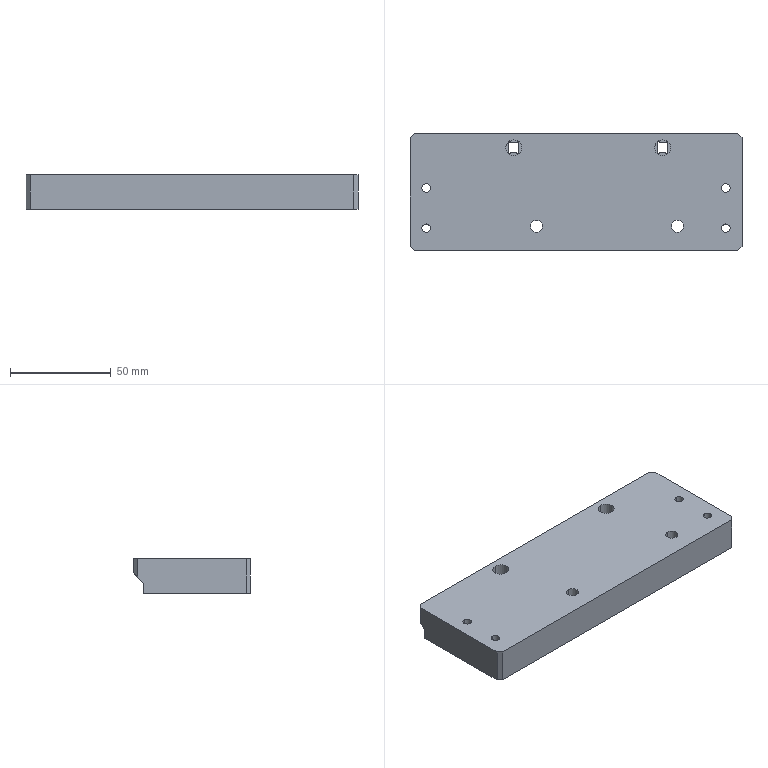NC program | NX | posted with a generic post | part box 165 x 58 x 17 mm
Lines 1 to 1651 of 3780, first 1438 of 1635 lines:
N10 G17 G21 G94 G90
(FLOOR_WALL , TOOL : D80)
N12 T19 M6
N14 G54
N16 G17 G0 G90 X127.5 Y0. S6500 M3
N18 G43 Z30. H19
N20 Z3.
N22 G94 G1 Z0. F1500.
N24 X124.5
N26 X-124.5
N28 X-127.5
N30 Z3.
N32 G0 Z30.
N34 M5
(ZLEVEL_PROFILE , TOOL : D10)
N36 T15 M6
N38 G54
N40 G17 G0 G90 X-47.703 Y34.1 S9500 M3
N42 G43 Z30. H15
N44 Z1.5
N46 G94 G1 X0. Z-1. F1000.
N48 X80.5 F3000.
N50 G2 X84.106 Y32.606 R5.1
N52 G1 X86.106 Y30.606
N54 G2 X87.6 Y27. R5.1
N56 G1 Y-27.
N58 G2 X86.106 Y-30.606 R5.1
N60 G1 X84.106 Y-32.606
N62 G2 X80.5 Y-34.1 R5.1
N64 G1 X-80.5
N66 G2 X-84.106 Y-32.606 R5.1
N68 G1 X-86.106 Y-30.606
N70 G2 X-87.6 Y-27. R5.1
N72 G1 Y27.
N74 G2 X-86.106 Y30.606 R5.1
N76 G1 X-84.106 Y32.606
N78 G2 X-80.5 Y34.1 R5.1
N80 G1 X0.
N82 X80.5 Z-1.17
N84 X81. Y34.075 Z-1.171
N86 X81.495 Y34.002 Z-1.172
N88 X81.98 Y33.88 Z-1.173
N90 X82.452 Y33.712 Z-1.174
N92 X82.904 Y33.498 Z-1.175
N94 X83.333 Y33.24 Z-1.176
N96 X83.735 Y32.942 Z-1.177
N98 X84.106 Y32.606 Z-1.179
N100 X86.106 Y30.606 Z-1.185
N102 X86.442 Y30.235 Z-1.186
N104 X86.74 Y29.833 Z-1.187
N106 X86.998 Y29.404 Z-1.188
N108 X87.212 Y28.952 Z-1.189
N110 X87.38 Y28.48 Z-1.19
N112 X87.502 Y27.995 Z-1.191
N114 X87.575 Y27.5 Z-1.192
N116 X87.6 Y27. Z-1.193
N118 Y-27. Z-1.307
N120 X87.575 Y-27.5 Z-1.308
N122 X87.502 Y-27.995 Z-1.309
N124 X87.38 Y-28.48 Z-1.31
N126 X87.212 Y-28.952 Z-1.311
N128 X86.998 Y-29.404 Z-1.312
N130 X86.74 Y-29.833 Z-1.313
N132 X86.442 Y-30.235 Z-1.314
N134 X86.106 Y-30.606 Z-1.315
N136 X84.106 Y-32.606 Z-1.321
N138 X83.735 Y-32.942 Z-1.323
N140 X83.333 Y-33.24 Z-1.324
N142 X82.904 Y-33.498 Z-1.325
N144 X82.452 Y-33.712 Z-1.326
N146 X81.98 Y-33.88 Z-1.327
N148 X81.495 Y-34.002 Z-1.328
N150 X81. Y-34.075 Z-1.329
N152 X80.5 Y-34.1 Z-1.33
N154 X-80.5 Z-1.67
N156 X-81. Y-34.075 Z-1.671
N158 X-81.495 Y-34.002 Z-1.672
N160 X-81.98 Y-33.88 Z-1.673
N162 X-82.452 Y-33.712 Z-1.674
N164 X-82.904 Y-33.498 Z-1.675
N166 X-83.333 Y-33.24 Z-1.676
N168 X-83.735 Y-32.942 Z-1.677
N170 X-84.106 Y-32.606 Z-1.679
N172 X-86.106 Y-30.606 Z-1.685
N174 X-86.442 Y-30.235 Z-1.686
N176 X-86.74 Y-29.833 Z-1.687
N178 X-86.998 Y-29.404 Z-1.688
N180 X-87.212 Y-28.952 Z-1.689
N182 X-87.38 Y-28.48 Z-1.69
N184 X-87.502 Y-27.995 Z-1.691
N186 X-87.575 Y-27.5 Z-1.692
N188 X-87.6 Y-27. Z-1.693
N190 Y27. Z-1.807
N192 X-87.575 Y27.5 Z-1.808
N194 X-87.502 Y27.995 Z-1.809
N196 X-87.38 Y28.48 Z-1.81
N198 X-87.212 Y28.952 Z-1.811
N200 X-86.998 Y29.404 Z-1.812
N202 X-86.74 Y29.833 Z-1.813
N204 X-86.442 Y30.235 Z-1.814
N206 X-86.106 Y30.606 Z-1.815
N208 X-84.106 Y32.606 Z-1.821
N210 X-83.735 Y32.942 Z-1.823
N212 X-83.333 Y33.24 Z-1.824
N214 X-82.904 Y33.498 Z-1.825
N216 X-82.452 Y33.712 Z-1.826
N218 X-81.98 Y33.88 Z-1.827
N220 X-81.495 Y34.002 Z-1.828
N222 X-81. Y34.075 Z-1.829
N224 X-80.5 Y34.1 Z-1.83
N226 X0. Z-2.
N228 X80.5 Z-2.17
N230 X81. Y34.075 Z-2.171
N232 X81.495 Y34.002 Z-2.172
N234 X81.98 Y33.88 Z-2.173
N236 X82.452 Y33.712 Z-2.174
N238 X82.904 Y33.498 Z-2.175
N240 X83.333 Y33.24 Z-2.176
N242 X83.735 Y32.942 Z-2.177
N244 X84.106 Y32.606 Z-2.179
N246 X86.106 Y30.606 Z-2.185
N248 X86.442 Y30.235 Z-2.186
N250 X86.74 Y29.833 Z-2.187
N252 X86.998 Y29.404 Z-2.188
N254 X87.212 Y28.952 Z-2.189
N256 X87.38 Y28.48 Z-2.19
N258 X87.502 Y27.995 Z-2.191
N260 X87.575 Y27.5 Z-2.192
N262 X87.6 Y27. Z-2.193
N264 Y-27. Z-2.307
N266 X87.575 Y-27.5 Z-2.308
N268 X87.502 Y-27.995 Z-2.309
N270 X87.38 Y-28.48 Z-2.31
N272 X87.212 Y-28.952 Z-2.311
N274 X86.998 Y-29.404 Z-2.312
N276 X86.74 Y-29.833 Z-2.313
N278 X86.442 Y-30.235 Z-2.314
N280 X86.106 Y-30.606 Z-2.315
N282 X84.106 Y-32.606 Z-2.321
N284 X83.735 Y-32.942 Z-2.323
N286 X83.333 Y-33.24 Z-2.324
N288 X82.904 Y-33.498 Z-2.325
N290 X82.452 Y-33.712 Z-2.326
N292 X81.98 Y-33.88 Z-2.327
N294 X81.495 Y-34.002 Z-2.328
N296 X81. Y-34.075 Z-2.329
N298 X80.5 Y-34.1 Z-2.33
N300 X-80.5 Z-2.67
N302 X-81. Y-34.075 Z-2.671
N304 X-81.495 Y-34.002 Z-2.672
N306 X-81.98 Y-33.88 Z-2.673
N308 X-82.452 Y-33.712 Z-2.674
N310 X-82.904 Y-33.498 Z-2.675
N312 X-83.333 Y-33.24 Z-2.676
N314 X-83.735 Y-32.942 Z-2.677
N316 X-84.106 Y-32.606 Z-2.679
N318 X-86.106 Y-30.606 Z-2.685
N320 X-86.442 Y-30.235 Z-2.686
N322 X-86.74 Y-29.833 Z-2.687
N324 X-86.998 Y-29.404 Z-2.688
N326 X-87.212 Y-28.952 Z-2.689
N328 X-87.38 Y-28.48 Z-2.69
N330 X-87.502 Y-27.995 Z-2.691
N332 X-87.575 Y-27.5 Z-2.692
N334 X-87.6 Y-27. Z-2.693
N336 Y27. Z-2.807
N338 X-87.575 Y27.5 Z-2.808
N340 X-87.502 Y27.995 Z-2.809
N342 X-87.38 Y28.48 Z-2.81
N344 X-87.212 Y28.952 Z-2.811
N346 X-86.998 Y29.404 Z-2.812
N348 X-86.74 Y29.833 Z-2.813
N350 X-86.442 Y30.235 Z-2.814
N352 X-86.106 Y30.606 Z-2.815
N354 X-84.106 Y32.606 Z-2.821
N356 X-83.735 Y32.942 Z-2.823
N358 X-83.333 Y33.24 Z-2.824
N360 X-82.904 Y33.498 Z-2.825
N362 X-82.452 Y33.712 Z-2.826
N364 X-81.98 Y33.88 Z-2.827
N366 X-81.495 Y34.002 Z-2.828
N368 X-81. Y34.075 Z-2.829
N370 X-80.5 Y34.1 Z-2.83
N372 X0. Z-3.
N374 X80.5 Z-3.17
N376 X81. Y34.075 Z-3.171
N378 X81.495 Y34.002 Z-3.172
N380 X81.98 Y33.88 Z-3.173
N382 X82.452 Y33.712 Z-3.174
N384 X82.904 Y33.498 Z-3.175
N386 X83.333 Y33.24 Z-3.176
N388 X83.735 Y32.942 Z-3.177
N390 X84.106 Y32.606 Z-3.179
N392 X86.106 Y30.606 Z-3.185
N394 X86.442 Y30.235 Z-3.186
N396 X86.74 Y29.833 Z-3.187
N398 X86.998 Y29.404 Z-3.188
N400 X87.212 Y28.952 Z-3.189
N402 X87.38 Y28.48 Z-3.19
N404 X87.502 Y27.995 Z-3.191
N406 X87.575 Y27.5 Z-3.192
N408 X87.6 Y27. Z-3.193
N410 Y-27. Z-3.307
N412 X87.575 Y-27.5 Z-3.308
N414 X87.502 Y-27.995 Z-3.309
N416 X87.38 Y-28.48 Z-3.31
N418 X87.212 Y-28.952 Z-3.311
N420 X86.998 Y-29.404 Z-3.312
N422 X86.74 Y-29.833 Z-3.313
N424 X86.442 Y-30.235 Z-3.314
N426 X86.106 Y-30.606 Z-3.315
N428 X84.106 Y-32.606 Z-3.321
N430 X83.735 Y-32.942 Z-3.323
N432 X83.333 Y-33.24 Z-3.324
N434 X82.904 Y-33.498 Z-3.325
N436 X82.452 Y-33.712 Z-3.326
N438 X81.98 Y-33.88 Z-3.327
N440 X81.495 Y-34.002 Z-3.328
N442 X81. Y-34.075 Z-3.329
N444 X80.5 Y-34.1 Z-3.33
N446 X-80.5 Z-3.67
N448 X-81. Y-34.075 Z-3.671
N450 X-81.495 Y-34.002 Z-3.672
N452 X-81.98 Y-33.88 Z-3.673
N454 X-82.452 Y-33.712 Z-3.674
N456 X-82.904 Y-33.498 Z-3.675
N458 X-83.333 Y-33.24 Z-3.676
N460 X-83.735 Y-32.942 Z-3.677
N462 X-84.106 Y-32.606 Z-3.679
N464 X-86.106 Y-30.606 Z-3.685
N466 X-86.442 Y-30.235 Z-3.686
N468 X-86.74 Y-29.833 Z-3.687
N470 X-86.998 Y-29.404 Z-3.688
N472 X-87.212 Y-28.952 Z-3.689
N474 X-87.38 Y-28.48 Z-3.69
N476 X-87.502 Y-27.995 Z-3.691
N478 X-87.575 Y-27.5 Z-3.692
N480 X-87.6 Y-27. Z-3.693
N482 Y27. Z-3.807
N484 X-87.575 Y27.5 Z-3.808
N486 X-87.502 Y27.995 Z-3.809
N488 X-87.38 Y28.48 Z-3.81
N490 X-87.212 Y28.952 Z-3.811
N492 X-86.998 Y29.404 Z-3.812
N494 X-86.74 Y29.833 Z-3.813
N496 X-86.442 Y30.235 Z-3.814
N498 X-86.106 Y30.606 Z-3.815
N500 X-84.106 Y32.606 Z-3.821
N502 X-83.735 Y32.942 Z-3.823
N504 X-83.333 Y33.24 Z-3.824
N506 X-82.904 Y33.498 Z-3.825
N508 X-82.452 Y33.712 Z-3.826
N510 X-81.98 Y33.88 Z-3.827
N512 X-81.495 Y34.002 Z-3.828
N514 X-81. Y34.075 Z-3.829
N516 X-80.5 Y34.1 Z-3.83
N518 X0. Z-4.
N520 X80.5 Z-4.17
N522 X81. Y34.075 Z-4.171
N524 X81.495 Y34.002 Z-4.172
N526 X81.98 Y33.88 Z-4.173
N528 X82.452 Y33.712 Z-4.174
N530 X82.904 Y33.498 Z-4.175
N532 X83.333 Y33.24 Z-4.176
N534 X83.735 Y32.942 Z-4.177
N536 X84.106 Y32.606 Z-4.179
N538 X86.106 Y30.606 Z-4.185
N540 X86.442 Y30.235 Z-4.186
N542 X86.74 Y29.833 Z-4.187
N544 X86.998 Y29.404 Z-4.188
N546 X87.212 Y28.952 Z-4.189
N548 X87.38 Y28.48 Z-4.19
N550 X87.502 Y27.995 Z-4.191
N552 X87.575 Y27.5 Z-4.192
N554 X87.6 Y27. Z-4.193
N556 Y-27. Z-4.307
N558 X87.575 Y-27.5 Z-4.308
N560 X87.502 Y-27.995 Z-4.309
N562 X87.38 Y-28.48 Z-4.31
N564 X87.212 Y-28.952 Z-4.311
N566 X86.998 Y-29.404 Z-4.312
N568 X86.74 Y-29.833 Z-4.313
N570 X86.442 Y-30.235 Z-4.314
N572 X86.106 Y-30.606 Z-4.315
N574 X84.106 Y-32.606 Z-4.321
N576 X83.735 Y-32.942 Z-4.323
N578 X83.333 Y-33.24 Z-4.324
N580 X82.904 Y-33.498 Z-4.325
N582 X82.452 Y-33.712 Z-4.326
N584 X81.98 Y-33.88 Z-4.327
N586 X81.495 Y-34.002 Z-4.328
N588 X81. Y-34.075 Z-4.329
N590 X80.5 Y-34.1 Z-4.33
N592 X-80.5 Z-4.67
N594 X-81. Y-34.075 Z-4.671
N596 X-81.495 Y-34.002 Z-4.672
N598 X-81.98 Y-33.88 Z-4.673
N600 X-82.452 Y-33.712 Z-4.674
N602 X-82.904 Y-33.498 Z-4.675
N604 X-83.333 Y-33.24 Z-4.676
N606 X-83.735 Y-32.942 Z-4.677
N608 X-84.106 Y-32.606 Z-4.679
N610 X-86.106 Y-30.606 Z-4.685
N612 X-86.442 Y-30.235 Z-4.686
N614 X-86.74 Y-29.833 Z-4.687
N616 X-86.998 Y-29.404 Z-4.688
N618 X-87.212 Y-28.952 Z-4.689
N620 X-87.38 Y-28.48 Z-4.69
N622 X-87.502 Y-27.995 Z-4.691
N624 X-87.575 Y-27.5 Z-4.692
N626 X-87.6 Y-27. Z-4.693
N628 Y27. Z-4.807
N630 X-87.575 Y27.5 Z-4.808
N632 X-87.502 Y27.995 Z-4.809
N634 X-87.38 Y28.48 Z-4.81
N636 X-87.212 Y28.952 Z-4.811
N638 X-86.998 Y29.404 Z-4.812
N640 X-86.74 Y29.833 Z-4.813
N642 X-86.442 Y30.235 Z-4.814
N644 X-86.106 Y30.606 Z-4.815
N646 X-84.106 Y32.606 Z-4.821
N648 X-83.735 Y32.942 Z-4.823
N650 X-83.333 Y33.24 Z-4.824
N652 X-82.904 Y33.498 Z-4.825
N654 X-82.452 Y33.712 Z-4.826
N656 X-81.98 Y33.88 Z-4.827
N658 X-81.495 Y34.002 Z-4.828
N660 X-81. Y34.075 Z-4.829
N662 X-80.5 Y34.1 Z-4.83
N664 X0. Z-5.
N666 X80.5 Z-5.17
N668 X81. Y34.075 Z-5.171
N670 X81.495 Y34.002 Z-5.172
N672 X81.98 Y33.88 Z-5.173
N674 X82.452 Y33.712 Z-5.174
N676 X82.904 Y33.498 Z-5.175
N678 X83.333 Y33.24 Z-5.176
N680 X83.735 Y32.942 Z-5.177
N682 X84.106 Y32.606 Z-5.179
N684 X86.106 Y30.606 Z-5.185
N686 X86.442 Y30.235 Z-5.186
N688 X86.74 Y29.833 Z-5.187
N690 X86.998 Y29.404 Z-5.188
N692 X87.212 Y28.952 Z-5.189
N694 X87.38 Y28.48 Z-5.19
N696 X87.502 Y27.995 Z-5.191
N698 X87.575 Y27.5 Z-5.192
N700 X87.6 Y27. Z-5.193
N702 Y-27. Z-5.307
N704 X87.575 Y-27.5 Z-5.308
N706 X87.502 Y-27.995 Z-5.309
N708 X87.38 Y-28.48 Z-5.31
N710 X87.212 Y-28.952 Z-5.311
N712 X86.998 Y-29.404 Z-5.312
N714 X86.74 Y-29.833 Z-5.313
N716 X86.442 Y-30.235 Z-5.314
N718 X86.106 Y-30.606 Z-5.315
N720 X84.106 Y-32.606 Z-5.321
N722 X83.735 Y-32.942 Z-5.323
N724 X83.333 Y-33.24 Z-5.324
N726 X82.904 Y-33.498 Z-5.325
N728 X82.452 Y-33.712 Z-5.326
N730 X81.98 Y-33.88 Z-5.327
N732 X81.495 Y-34.002 Z-5.328
N734 X81. Y-34.075 Z-5.329
N736 X80.5 Y-34.1 Z-5.33
N738 X-80.5 Z-5.67
N740 X-81. Y-34.075 Z-5.671
N742 X-81.495 Y-34.002 Z-5.672
N744 X-81.98 Y-33.88 Z-5.673
N746 X-82.452 Y-33.712 Z-5.674
N748 X-82.904 Y-33.498 Z-5.675
N750 X-83.333 Y-33.24 Z-5.676
N752 X-83.735 Y-32.942 Z-5.677
N754 X-84.106 Y-32.606 Z-5.679
N756 X-86.106 Y-30.606 Z-5.685
N758 X-86.442 Y-30.235 Z-5.686
N760 X-86.74 Y-29.833 Z-5.687
N762 X-86.998 Y-29.404 Z-5.688
N764 X-87.212 Y-28.952 Z-5.689
N766 X-87.38 Y-28.48 Z-5.69
N768 X-87.502 Y-27.995 Z-5.691
N770 X-87.575 Y-27.5 Z-5.692
N772 X-87.6 Y-27. Z-5.693
N774 Y27. Z-5.807
N776 X-87.575 Y27.5 Z-5.808
N778 X-87.502 Y27.995 Z-5.809
N780 X-87.38 Y28.48 Z-5.81
N782 X-87.212 Y28.952 Z-5.811
N784 X-86.998 Y29.404 Z-5.812
N786 X-86.74 Y29.833 Z-5.813
N788 X-86.442 Y30.235 Z-5.814
N790 X-86.106 Y30.606 Z-5.815
N792 X-84.106 Y32.606 Z-5.821
N794 X-83.735 Y32.942 Z-5.823
N796 X-83.333 Y33.24 Z-5.824
N798 X-82.904 Y33.498 Z-5.825
N800 X-82.452 Y33.712 Z-5.826
N802 X-81.98 Y33.88 Z-5.827
N804 X-81.495 Y34.002 Z-5.828
N806 X-81. Y34.075 Z-5.829
N808 X-80.5 Y34.1 Z-5.83
N810 X0. Z-6.
N812 X80.5 Z-6.17
N814 X81. Y34.075 Z-6.171
N816 X81.495 Y34.002 Z-6.172
N818 X81.98 Y33.88 Z-6.173
N820 X82.452 Y33.712 Z-6.174
N822 X82.904 Y33.498 Z-6.175
N824 X83.333 Y33.24 Z-6.176
N826 X83.735 Y32.942 Z-6.177
N828 X84.106 Y32.606 Z-6.179
N830 X86.106 Y30.606 Z-6.185
N832 X86.442 Y30.235 Z-6.186
N834 X86.74 Y29.833 Z-6.187
N836 X86.998 Y29.404 Z-6.188
N838 X87.212 Y28.952 Z-6.189
N840 X87.38 Y28.48 Z-6.19
N842 X87.502 Y27.995 Z-6.191
N844 X87.575 Y27.5 Z-6.192
N846 X87.6 Y27. Z-6.193
N848 Y-27. Z-6.307
N850 X87.575 Y-27.5 Z-6.308
N852 X87.502 Y-27.995 Z-6.309
N854 X87.38 Y-28.48 Z-6.31
N856 X87.212 Y-28.952 Z-6.311
N858 X86.998 Y-29.404 Z-6.312
N860 X86.74 Y-29.833 Z-6.313
N862 X86.442 Y-30.235 Z-6.314
N864 X86.106 Y-30.606 Z-6.315
N866 X84.106 Y-32.606 Z-6.321
N868 X83.735 Y-32.942 Z-6.323
N870 X83.333 Y-33.24 Z-6.324
N872 X82.904 Y-33.498 Z-6.325
N874 X82.452 Y-33.712 Z-6.326
N876 X81.98 Y-33.88 Z-6.327
N878 X81.495 Y-34.002 Z-6.328
N880 X81. Y-34.075 Z-6.329
N882 X80.5 Y-34.1 Z-6.33
N884 X-80.5 Z-6.67
N886 X-81. Y-34.075 Z-6.671
N888 X-81.495 Y-34.002 Z-6.672
N890 X-81.98 Y-33.88 Z-6.673
N892 X-82.452 Y-33.712 Z-6.674
N894 X-82.904 Y-33.498 Z-6.675
N896 X-83.333 Y-33.24 Z-6.676
N898 X-83.735 Y-32.942 Z-6.677
N900 X-84.106 Y-32.606 Z-6.679
N902 X-86.106 Y-30.606 Z-6.685
N904 X-86.442 Y-30.235 Z-6.686
N906 X-86.74 Y-29.833 Z-6.687
N908 X-86.998 Y-29.404 Z-6.688
N910 X-87.212 Y-28.952 Z-6.689
N912 X-87.38 Y-28.48 Z-6.69
N914 X-87.502 Y-27.995 Z-6.691
N916 X-87.575 Y-27.5 Z-6.692
N918 X-87.6 Y-27. Z-6.693
N920 Y27. Z-6.807
N922 X-87.575 Y27.5 Z-6.808
N924 X-87.502 Y27.995 Z-6.809
N926 X-87.38 Y28.48 Z-6.81
N928 X-87.212 Y28.952 Z-6.811
N930 X-86.998 Y29.404 Z-6.812
N932 X-86.74 Y29.833 Z-6.813
N934 X-86.442 Y30.235 Z-6.814
N936 X-86.106 Y30.606 Z-6.815
N938 X-84.106 Y32.606 Z-6.821
N940 X-83.735 Y32.942 Z-6.823
N942 X-83.333 Y33.24 Z-6.824
N944 X-82.904 Y33.498 Z-6.825
N946 X-82.452 Y33.712 Z-6.826
N948 X-81.98 Y33.88 Z-6.827
N950 X-81.495 Y34.002 Z-6.828
N952 X-81. Y34.075 Z-6.829
N954 X-80.5 Y34.1 Z-6.83
N956 X0. Z-7.
N958 X80.5 Z-7.17
N960 X81. Y34.075 Z-7.171
N962 X81.495 Y34.002 Z-7.172
N964 X81.98 Y33.88 Z-7.173
N966 X82.452 Y33.712 Z-7.174
N968 X82.904 Y33.498 Z-7.175
N970 X83.333 Y33.24 Z-7.176
N972 X83.735 Y32.942 Z-7.177
N974 X84.106 Y32.606 Z-7.179
N976 X86.106 Y30.606 Z-7.185
N978 X86.442 Y30.235 Z-7.186
N980 X86.74 Y29.833 Z-7.187
N982 X86.998 Y29.404 Z-7.188
N984 X87.212 Y28.952 Z-7.189
N986 X87.38 Y28.48 Z-7.19
N988 X87.502 Y27.995 Z-7.191
N990 X87.575 Y27.5 Z-7.192
N992 X87.6 Y27. Z-7.193
N994 Y-27. Z-7.307
N996 X87.575 Y-27.5 Z-7.308
N998 X87.502 Y-27.995 Z-7.309
N1000 X87.38 Y-28.48 Z-7.31
N1002 X87.212 Y-28.952 Z-7.311
N1004 X86.998 Y-29.404 Z-7.312
N1006 X86.74 Y-29.833 Z-7.313
N1008 X86.442 Y-30.235 Z-7.314
N1010 X86.106 Y-30.606 Z-7.315
N1012 X84.106 Y-32.606 Z-7.321
N1014 X83.735 Y-32.942 Z-7.323
N1016 X83.333 Y-33.24 Z-7.324
N1018 X82.904 Y-33.498 Z-7.325
N1020 X82.452 Y-33.712 Z-7.326
N1022 X81.98 Y-33.88 Z-7.327
N1024 X81.495 Y-34.002 Z-7.328
N1026 X81. Y-34.075 Z-7.329
N1028 X80.5 Y-34.1 Z-7.33
N1030 X-80.5 Z-7.67
N1032 X-81. Y-34.075 Z-7.671
N1034 X-81.495 Y-34.002 Z-7.672
N1036 X-81.98 Y-33.88 Z-7.673
N1038 X-82.452 Y-33.712 Z-7.674
N1040 X-82.904 Y-33.498 Z-7.675
N1042 X-83.333 Y-33.24 Z-7.676
N1044 X-83.735 Y-32.942 Z-7.677
N1046 X-84.106 Y-32.606 Z-7.679
N1048 X-86.106 Y-30.606 Z-7.685
N1050 X-86.442 Y-30.235 Z-7.686
N1052 X-86.74 Y-29.833 Z-7.687
N1054 X-86.998 Y-29.404 Z-7.688
N1056 X-87.212 Y-28.952 Z-7.689
N1058 X-87.38 Y-28.48 Z-7.69
N1060 X-87.502 Y-27.995 Z-7.691
N1062 X-87.575 Y-27.5 Z-7.692
N1064 X-87.6 Y-27. Z-7.693
N1066 Y27. Z-7.807
N1068 X-87.575 Y27.5 Z-7.808
N1070 X-87.502 Y27.995 Z-7.809
N1072 X-87.38 Y28.48 Z-7.81
N1074 X-87.212 Y28.952 Z-7.811
N1076 X-86.998 Y29.404 Z-7.812
N1078 X-86.74 Y29.833 Z-7.813
N1080 X-86.442 Y30.235 Z-7.814
N1082 X-86.106 Y30.606 Z-7.815
N1084 X-84.106 Y32.606 Z-7.821
N1086 X-83.735 Y32.942 Z-7.823
N1088 X-83.333 Y33.24 Z-7.824
N1090 X-82.904 Y33.498 Z-7.825
N1092 X-82.452 Y33.712 Z-7.826
N1094 X-81.98 Y33.88 Z-7.827
N1096 X-81.495 Y34.002 Z-7.828
N1098 X-81. Y34.075 Z-7.829
N1100 X-80.5 Y34.1 Z-7.83
N1102 X0. Z-8.
N1104 X80.5 Z-8.17
N1106 X81. Y34.075 Z-8.171
N1108 X81.495 Y34.002 Z-8.172
N1110 X81.98 Y33.88 Z-8.173
N1112 X82.452 Y33.712 Z-8.174
N1114 X82.904 Y33.498 Z-8.175
N1116 X83.333 Y33.24 Z-8.176
N1118 X83.735 Y32.942 Z-8.177
N1120 X84.106 Y32.606 Z-8.179
N1122 X86.106 Y30.606 Z-8.185
N1124 X86.442 Y30.235 Z-8.186
N1126 X86.74 Y29.833 Z-8.187
N1128 X86.998 Y29.404 Z-8.188
N1130 X87.212 Y28.952 Z-8.189
N1132 X87.38 Y28.48 Z-8.19
N1134 X87.502 Y27.995 Z-8.191
N1136 X87.575 Y27.5 Z-8.192
N1138 X87.6 Y27. Z-8.193
N1140 Y-27. Z-8.307
N1142 X87.575 Y-27.5 Z-8.308
N1144 X87.502 Y-27.995 Z-8.309
N1146 X87.38 Y-28.48 Z-8.31
N1148 X87.212 Y-28.952 Z-8.311
N1150 X86.998 Y-29.404 Z-8.312
N1152 X86.74 Y-29.833 Z-8.313
N1154 X86.442 Y-30.235 Z-8.314
N1156 X86.106 Y-30.606 Z-8.315
N1158 X84.106 Y-32.606 Z-8.321
N1160 X83.735 Y-32.942 Z-8.323
N1162 X83.333 Y-33.24 Z-8.324
N1164 X82.904 Y-33.498 Z-8.325
N1166 X82.452 Y-33.712 Z-8.326
N1168 X81.98 Y-33.88 Z-8.327
N1170 X81.495 Y-34.002 Z-8.328
N1172 X81. Y-34.075 Z-8.329
N1174 X80.5 Y-34.1 Z-8.33
N1176 X-80.5 Z-8.67
N1178 X-81. Y-34.075 Z-8.671
N1180 X-81.495 Y-34.002 Z-8.672
N1182 X-81.98 Y-33.88 Z-8.673
N1184 X-82.452 Y-33.712 Z-8.674
N1186 X-82.904 Y-33.498 Z-8.675
N1188 X-83.333 Y-33.24 Z-8.676
N1190 X-83.735 Y-32.942 Z-8.677
N1192 X-84.106 Y-32.606 Z-8.679
N1194 X-86.106 Y-30.606 Z-8.685
N1196 X-86.442 Y-30.235 Z-8.686
N1198 X-86.74 Y-29.833 Z-8.687
N1200 X-86.998 Y-29.404 Z-8.688
N1202 X-87.212 Y-28.952 Z-8.689
N1204 X-87.38 Y-28.48 Z-8.69
N1206 X-87.502 Y-27.995 Z-8.691
N1208 X-87.575 Y-27.5 Z-8.692
N1210 X-87.6 Y-27. Z-8.693
N1212 Y27. Z-8.807
N1214 X-87.575 Y27.5 Z-8.808
N1216 X-87.502 Y27.995 Z-8.809
N1218 X-87.38 Y28.48 Z-8.81
N1220 X-87.212 Y28.952 Z-8.811
N1222 X-86.998 Y29.404 Z-8.812
N1224 X-86.74 Y29.833 Z-8.813
N1226 X-86.442 Y30.235 Z-8.814
N1228 X-86.106 Y30.606 Z-8.815
N1230 X-84.106 Y32.606 Z-8.821
N1232 X-83.735 Y32.942 Z-8.823
N1234 X-83.333 Y33.24 Z-8.824
N1236 X-82.904 Y33.498 Z-8.825
N1238 X-82.452 Y33.712 Z-8.826
N1240 X-81.98 Y33.88 Z-8.827
N1242 X-81.495 Y34.002 Z-8.828
N1244 X-81. Y34.075 Z-8.829
N1246 X-80.5 Y34.1 Z-8.83
N1248 X0. Z-9.
N1250 X80.5 Z-9.17
N1252 X81. Y34.075 Z-9.171
N1254 X81.495 Y34.002 Z-9.172
N1256 X81.98 Y33.88 Z-9.173
N1258 X82.452 Y33.712 Z-9.174
N1260 X82.904 Y33.498 Z-9.175
N1262 X83.333 Y33.24 Z-9.176
N1264 X83.735 Y32.942 Z-9.177
N1266 X84.106 Y32.606 Z-9.179
N1268 X86.106 Y30.606 Z-9.185
N1270 X86.442 Y30.235 Z-9.186
N1272 X86.74 Y29.833 Z-9.187
N1274 X86.998 Y29.404 Z-9.188
N1276 X87.212 Y28.952 Z-9.189
N1278 X87.38 Y28.48 Z-9.19
N1280 X87.502 Y27.995 Z-9.191
N1282 X87.575 Y27.5 Z-9.192
N1284 X87.6 Y27. Z-9.193
N1286 Y-27. Z-9.307
N1288 X87.575 Y-27.5 Z-9.308
N1290 X87.502 Y-27.995 Z-9.309
N1292 X87.38 Y-28.48 Z-9.31
N1294 X87.212 Y-28.952 Z-9.311
N1296 X86.998 Y-29.404 Z-9.312
N1298 X86.74 Y-29.833 Z-9.313
N1300 X86.442 Y-30.235 Z-9.314
N1302 X86.106 Y-30.606 Z-9.315
N1304 X84.106 Y-32.606 Z-9.321
N1306 X83.735 Y-32.942 Z-9.323
N1308 X83.333 Y-33.24 Z-9.324
N1310 X82.904 Y-33.498 Z-9.325
N1312 X82.452 Y-33.712 Z-9.326
N1314 X81.98 Y-33.88 Z-9.327
N1316 X81.495 Y-34.002 Z-9.328
N1318 X81. Y-34.075 Z-9.329
N1320 X80.5 Y-34.1 Z-9.33
N1322 X-80.5 Z-9.67
N1324 X-81. Y-34.075 Z-9.671
N1326 X-81.495 Y-34.002 Z-9.672
N1328 X-81.98 Y-33.88 Z-9.673
N1330 X-82.452 Y-33.712 Z-9.674
N1332 X-82.904 Y-33.498 Z-9.675
N1334 X-83.333 Y-33.24 Z-9.676
N1336 X-83.735 Y-32.942 Z-9.677
N1338 X-84.106 Y-32.606 Z-9.679
N1340 X-86.106 Y-30.606 Z-9.685
N1342 X-86.442 Y-30.235 Z-9.686
N1344 X-86.74 Y-29.833 Z-9.687
N1346 X-86.998 Y-29.404 Z-9.688
N1348 X-87.212 Y-28.952 Z-9.689
N1350 X-87.38 Y-28.48 Z-9.69
N1352 X-87.502 Y-27.995 Z-9.691
N1354 X-87.575 Y-27.5 Z-9.692
N1356 X-87.6 Y-27. Z-9.693
N1358 Y27. Z-9.807
N1360 X-87.575 Y27.5 Z-9.808
N1362 X-87.502 Y27.995 Z-9.809
N1364 X-87.38 Y28.48 Z-9.81
N1366 X-87.212 Y28.952 Z-9.811
N1368 X-86.998 Y29.404 Z-9.812
N1370 X-86.74 Y29.833 Z-9.813
N1372 X-86.442 Y30.235 Z-9.814
N1374 X-86.106 Y30.606 Z-9.815
N1376 X-84.106 Y32.606 Z-9.821
N1378 X-83.735 Y32.942 Z-9.823
N1380 X-83.333 Y33.24 Z-9.824
N1382 X-82.904 Y33.498 Z-9.825
N1384 X-82.452 Y33.712 Z-9.826
N1386 X-81.98 Y33.88 Z-9.827
N1388 X-81.495 Y34.002 Z-9.828
N1390 X-81. Y34.075 Z-9.829
N1392 X-80.5 Y34.1 Z-9.83
N1394 X0. Z-10.
N1396 X80.5 Z-10.17
N1398 X81. Y34.075 Z-10.171
N1400 X81.495 Y34.002 Z-10.172
N1402 X81.98 Y33.88 Z-10.173
N1404 X82.452 Y33.712 Z-10.174
N1406 X82.904 Y33.498 Z-10.175
N1408 X83.333 Y33.24 Z-10.176
N1410 X83.735 Y32.942 Z-10.177
N1412 X84.106 Y32.606 Z-10.179
N1414 X86.106 Y30.606 Z-10.185
N1416 X86.442 Y30.235 Z-10.186
N1418 X86.74 Y29.833 Z-10.187
N1420 X86.998 Y29.404 Z-10.188
N1422 X87.212 Y28.952 Z-10.189
N1424 X87.38 Y28.48 Z-10.19
N1426 X87.502 Y27.995 Z-10.191
N1428 X87.575 Y27.5 Z-10.192
N1430 X87.6 Y27. Z-10.193
N1432 Y-27. Z-10.307
N1434 X87.575 Y-27.5 Z-10.308
N1436 X87.502 Y-27.995 Z-10.309
N1438 X87.38 Y-28.48 Z-10.31
N1440 X87.212 Y-28.952 Z-10.311
N1442 X86.998 Y-29.404 Z-10.312
N1444 X86.74 Y-29.833 Z-10.313
N1446 X86.442 Y-30.235 Z-10.314
N1448 X86.106 Y-30.606 Z-10.315
N1450 X84.106 Y-32.606 Z-10.321
N1452 X83.735 Y-32.942 Z-10.323
N1454 X83.333 Y-33.24 Z-10.324
N1456 X82.904 Y-33.498 Z-10.325
N1458 X82.452 Y-33.712 Z-10.326
N1460 X81.98 Y-33.88 Z-10.327
N1462 X81.495 Y-34.002 Z-10.328
N1464 X81. Y-34.075 Z-10.329
N1466 X80.5 Y-34.1 Z-10.33
N1468 X-80.5 Z-10.67
N1470 X-81. Y-34.075 Z-10.671
N1472 X-81.495 Y-34.002 Z-10.672
N1474 X-81.98 Y-33.88 Z-10.673
N1476 X-82.452 Y-33.712 Z-10.674
N1478 X-82.904 Y-33.498 Z-10.675
N1480 X-83.333 Y-33.24 Z-10.676
N1482 X-83.735 Y-32.942 Z-10.677
N1484 X-84.106 Y-32.606 Z-10.679
N1486 X-86.106 Y-30.606 Z-10.685
N1488 X-86.442 Y-30.235 Z-10.686
N1490 X-86.74 Y-29.833 Z-10.687
N1492 X-86.998 Y-29.404 Z-10.688
N1494 X-87.212 Y-28.952 Z-10.689
N1496 X-87.38 Y-28.48 Z-10.69
N1498 X-87.502 Y-27.995 Z-10.691
N1500 X-87.575 Y-27.5 Z-10.692
N1502 X-87.6 Y-27. Z-10.693
N1504 Y27. Z-10.807
N1506 X-87.575 Y27.5 Z-10.808
N1508 X-87.502 Y27.995 Z-10.809
N1510 X-87.38 Y28.48 Z-10.81
N1512 X-87.212 Y28.952 Z-10.811
N1514 X-86.998 Y29.404 Z-10.812
N1516 X-86.74 Y29.833 Z-10.813
N1518 X-86.442 Y30.235 Z-10.814
N1520 X-86.106 Y30.606 Z-10.815
N1522 X-84.106 Y32.606 Z-10.821
N1524 X-83.735 Y32.942 Z-10.823
N1526 X-83.333 Y33.24 Z-10.824
N1528 X-82.904 Y33.498 Z-10.825
N1530 X-82.452 Y33.712 Z-10.826
N1532 X-81.98 Y33.88 Z-10.827
N1534 X-81.495 Y34.002 Z-10.828
N1536 X-81. Y34.075 Z-10.829
N1538 X-80.5 Y34.1 Z-10.83
N1540 X0. Z-11.
N1542 X80.5 Z-11.17
N1544 X81. Y34.075 Z-11.171
N1546 X81.495 Y34.002 Z-11.172
N1548 X81.98 Y33.88 Z-11.173
N1550 X82.452 Y33.712 Z-11.174
N1552 X82.904 Y33.498 Z-11.175
N1554 X83.333 Y33.24 Z-11.176
N1556 X83.735 Y32.942 Z-11.177
N1558 X84.106 Y32.606 Z-11.179
N1560 X86.106 Y30.606 Z-11.185
N1562 X86.442 Y30.235 Z-11.186
N1564 X86.74 Y29.833 Z-11.187
N1566 X86.998 Y29.404 Z-11.188
N1568 X87.212 Y28.952 Z-11.189
N1570 X87.38 Y28.48 Z-11.19
N1572 X87.502 Y27.995 Z-11.191
N1574 X87.575 Y27.5 Z-11.192
N1576 X87.6 Y27. Z-11.193
N1578 Y-27. Z-11.307
N1580 X87.575 Y-27.5 Z-11.308
N1582 X87.502 Y-27.995 Z-11.309
N1584 X87.38 Y-28.48 Z-11.31
N1586 X87.212 Y-28.952 Z-11.311
N1588 X86.998 Y-29.404 Z-11.312
N1590 X86.74 Y-29.833 Z-11.313
N1592 X86.442 Y-30.235 Z-11.314
N1594 X86.106 Y-30.606 Z-11.315
N1596 X84.106 Y-32.606 Z-11.321
N1598 X83.735 Y-32.942 Z-11.323
N1600 X83.333 Y-33.24 Z-11.324
N1602 X82.904 Y-33.498 Z-11.325
N1604 X82.452 Y-33.712 Z-11.326
N1606 X81.98 Y-33.88 Z-11.327
N1608 X81.495 Y-34.002 Z-11.328
N1610 X81. Y-34.075 Z-11.329
N1612 X80.5 Y-34.1 Z-11.33
N1614 X-80.5 Z-11.67
N1616 X-81. Y-34.075 Z-11.671
N1618 X-81.495 Y-34.002 Z-11.672
N1620 X-81.98 Y-33.88 Z-11.673
N1622 X-82.452 Y-33.712 Z-11.674
N1624 X-82.904 Y-33.498 Z-11.675
N1626 X-83.333 Y-33.24 Z-11.676
N1628 X-83.735 Y-32.942 Z-11.677
N1630 X-84.106 Y-32.606 Z-11.679
N1632 X-86.106 Y-30.606 Z-11.685
N1634 X-86.442 Y-30.235 Z-11.686
N1636 X-86.74 Y-29.833 Z-11.687
N1638 X-86.998 Y-29.404 Z-11.688
N1640 X-87.212 Y-28.952 Z-11.689
N1642 X-87.38 Y-28.48 Z-11.69
N1644 X-87.502 Y-27.995 Z-11.691
N1646 X-87.575 Y-27.5 Z-11.692
N1648 X-87.6 Y-27. Z-11.693
N1650 Y27. Z-11.807
N1652 X-87.575 Y27.5 Z-11.808
N1654 X-87.502 Y27.995 Z-11.809
N1656 X-87.38 Y28.48 Z-11.81
N1658 X-87.212 Y28.952 Z-11.811
N1660 X-86.998 Y29.404 Z-11.812
N1662 X-86.74 Y29.833 Z-11.813
N1664 X-86.442 Y30.235 Z-11.814
N1666 X-86.106 Y30.606 Z-11.815
N1668 X-84.106 Y32.606 Z-11.821
N1670 X-83.735 Y32.942 Z-11.823
N1672 X-83.333 Y33.24 Z-11.824
N1674 X-82.904 Y33.498 Z-11.825
N1676 X-82.452 Y33.712 Z-11.826
N1678 X-81.98 Y33.88 Z-11.827
N1680 X-81.495 Y34.002 Z-11.828
N1682 X-81. Y34.075 Z-11.829
N1684 X-80.5 Y34.1 Z-11.83
N1686 X0. Z-12.
N1688 X80.5 Z-12.17
N1690 X81. Y34.075 Z-12.171
N1692 X81.495 Y34.002 Z-12.172
N1694 X81.98 Y33.88 Z-12.173
N1696 X82.452 Y33.712 Z-12.174
N1698 X82.904 Y33.498 Z-12.175
N1700 X83.333 Y33.24 Z-12.176
N1702 X83.735 Y32.942 Z-12.177
N1704 X84.106 Y32.606 Z-12.179
N1706 X86.106 Y30.606 Z-12.185
N1708 X86.442 Y30.235 Z-12.186
N1710 X86.74 Y29.833 Z-12.187
N1712 X86.998 Y29.404 Z-12.188
N1714 X87.212 Y28.952 Z-12.189
N1716 X87.38 Y28.48 Z-12.19
N1718 X87.502 Y27.995 Z-12.191
N1720 X87.575 Y27.5 Z-12.192
N1722 X87.6 Y27. Z-12.193
N1724 Y-27. Z-12.307
N1726 X87.575 Y-27.5 Z-12.308
N1728 X87.502 Y-27.995 Z-12.309
N1730 X87.38 Y-28.48 Z-12.31
N1732 X87.212 Y-28.952 Z-12.311
N1734 X86.998 Y-29.404 Z-12.312
N1736 X86.74 Y-29.833 Z-12.313
N1738 X86.442 Y-30.235 Z-12.314
N1740 X86.106 Y-30.606 Z-12.315
N1742 X84.106 Y-32.606 Z-12.321
N1744 X83.735 Y-32.942 Z-12.323
N1746 X83.333 Y-33.24 Z-12.324
N1748 X82.904 Y-33.498 Z-12.325
N1750 X82.452 Y-33.712 Z-12.326
N1752 X81.98 Y-33.88 Z-12.327
N1754 X81.495 Y-34.002 Z-12.328
N1756 X81. Y-34.075 Z-12.329
N1758 X80.5 Y-34.1 Z-12.33
N1760 X-80.5 Z-12.67
N1762 X-81. Y-34.075 Z-12.671
N1764 X-81.495 Y-34.002 Z-12.672
N1766 X-81.98 Y-33.88 Z-12.673
N1768 X-82.452 Y-33.712 Z-12.674
N1770 X-82.904 Y-33.498 Z-12.675
N1772 X-83.333 Y-33.24 Z-12.676
N1774 X-83.735 Y-32.942 Z-12.677
N1776 X-84.106 Y-32.606 Z-12.679
N1778 X-86.106 Y-30.606 Z-12.685
N1780 X-86.442 Y-30.235 Z-12.686
N1782 X-86.74 Y-29.833 Z-12.687
N1784 X-86.998 Y-29.404 Z-12.688
N1786 X-87.212 Y-28.952 Z-12.689
N1788 X-87.38 Y-28.48 Z-12.69
N1790 X-87.502 Y-27.995 Z-12.691
N1792 X-87.575 Y-27.5 Z-12.692
N1794 X-87.6 Y-27. Z-12.693
N1796 Y27. Z-12.807
N1798 X-87.575 Y27.5 Z-12.808
N1800 X-87.502 Y27.995 Z-12.809
N1802 X-87.38 Y28.48 Z-12.81
N1804 X-87.212 Y28.952 Z-12.811
N1806 X-86.998 Y29.404 Z-12.812
N1808 X-86.74 Y29.833 Z-12.813
N1810 X-86.442 Y30.235 Z-12.814
N1812 X-86.106 Y30.606 Z-12.815
N1814 X-84.106 Y32.606 Z-12.821
N1816 X-83.735 Y32.942 Z-12.823
N1818 X-83.333 Y33.24 Z-12.824
N1820 X-82.904 Y33.498 Z-12.825
N1822 X-82.452 Y33.712 Z-12.826
N1824 X-81.98 Y33.88 Z-12.827
N1826 X-81.495 Y34.002 Z-12.828
N1828 X-81. Y34.075 Z-12.829
N1830 X-80.5 Y34.1 Z-12.83
N1832 X0. Z-13.
N1834 X80.5 Z-13.17
N1836 X81. Y34.075 Z-13.171
N1838 X81.495 Y34.002 Z-13.172
N1840 X81.98 Y33.88 Z-13.173
N1842 X82.452 Y33.712 Z-13.174
N1844 X82.904 Y33.498 Z-13.175
N1846 X83.333 Y33.24 Z-13.176
N1848 X83.735 Y32.942 Z-13.177
N1850 X84.106 Y32.606 Z-13.179
N1852 X86.106 Y30.606 Z-13.185
N1854 X86.442 Y30.235 Z-13.186
N1856 X86.74 Y29.833 Z-13.187
N1858 X86.998 Y29.404 Z-13.188
N1860 X87.212 Y28.952 Z-13.189
N1862 X87.38 Y28.48 Z-13.19
N1864 X87.502 Y27.995 Z-13.191
N1866 X87.575 Y27.5 Z-13.192
N1868 X87.6 Y27. Z-13.193
N1870 Y-27. Z-13.307
N1872 X87.575 Y-27.5 Z-13.308
N1874 X87.502 Y-27.995 Z-13.309
N1876 X87.38 Y-28.48 Z-13.31
N1878 X87.212 Y-28.952 Z-13.311
N1880 X86.998 Y-29.404 Z-13.312
N1882 X86.74 Y-29.833 Z-13.313
N1884 X86.442 Y-30.235 Z-13.314
N1886 X86.106 Y-30.606 Z-13.315
N1888 X84.106 Y-32.606 Z-13.321
N1890 X83.735 Y-32.942 Z-13.323
N1892 X83.333 Y-33.24 Z-13.324
N1894 X82.904 Y-33.498 Z-13.325
N1896 X82.452 Y-33.712 Z-13.326
N1898 X81.98 Y-33.88 Z-13.327
N1900 X81.495 Y-34.002 Z-13.328
N1902 X81. Y-34.075 Z-13.329
N1904 X80.5 Y-34.1 Z-13.33
N1906 X-80.5 Z-13.67
N1908 X-81. Y-34.075 Z-13.671
N1910 X-81.495 Y-34.002 Z-13.672
N1912 X-81.98 Y-33.88 Z-13.673
N1914 X-82.452 Y-33.712 Z-13.674
N1916 X-82.904 Y-33.498 Z-13.675
N1918 X-83.333 Y-33.24 Z-13.676
N1920 X-83.735 Y-32.942 Z-13.677
N1922 X-84.106 Y-32.606 Z-13.679
N1924 X-86.106 Y-30.606 Z-13.685
N1926 X-86.442 Y-30.235 Z-13.686
N1928 X-86.74 Y-29.833 Z-13.687
N1930 X-86.998 Y-29.404 Z-13.688
N1932 X-87.212 Y-28.952 Z-13.689
N1934 X-87.38 Y-28.48 Z-13.69
N1936 X-87.502 Y-27.995 Z-13.691
N1938 X-87.575 Y-27.5 Z-13.692
N1940 X-87.6 Y-27. Z-13.693
N1942 Y27. Z-13.807
N1944 X-87.575 Y27.5 Z-13.808
N1946 X-87.502 Y27.995 Z-13.809
N1948 X-87.38 Y28.48 Z-13.81
N1950 X-87.212 Y28.952 Z-13.811
N1952 X-86.998 Y29.404 Z-13.812
N1954 X-86.74 Y29.833 Z-13.813
N1956 X-86.442 Y30.235 Z-13.814
N1958 X-86.106 Y30.606 Z-13.815
N1960 X-84.106 Y32.606 Z-13.821
N1962 X-83.735 Y32.942 Z-13.823
N1964 X-83.333 Y33.24 Z-13.824
N1966 X-82.904 Y33.498 Z-13.825
N1968 X-82.452 Y33.712 Z-13.826
N1970 X-81.98 Y33.88 Z-13.827
N1972 X-81.495 Y34.002 Z-13.828
N1974 X-81. Y34.075 Z-13.829
N1976 X-80.5 Y34.1 Z-13.83
N1978 X0. Z-14.
N1980 X80.5 Z-14.17
N1982 X81. Y34.075 Z-14.171
N1984 X81.495 Y34.002 Z-14.172
N1986 X81.98 Y33.88 Z-14.173
N1988 X82.452 Y33.712 Z-14.174
N1990 X82.904 Y33.498 Z-14.175
N1992 X83.333 Y33.24 Z-14.176
N1994 X83.735 Y32.942 Z-14.177
N1996 X84.106 Y32.606 Z-14.179
N1998 X86.106 Y30.606 Z-14.185
N2000 X86.442 Y30.235 Z-14.186
N2002 X86.74 Y29.833 Z-14.187
N2004 X86.998 Y29.404 Z-14.188
N2006 X87.212 Y28.952 Z-14.189
N2008 X87.38 Y28.48 Z-14.19
N2010 X87.502 Y27.995 Z-14.191
N2012 X87.575 Y27.5 Z-14.192
N2014 X87.6 Y27. Z-14.193
N2016 Y-27. Z-14.307
N2018 X87.575 Y-27.5 Z-14.308
N2020 X87.502 Y-27.995 Z-14.309
N2022 X87.38 Y-28.48 Z-14.31
N2024 X87.212 Y-28.952 Z-14.311
N2026 X86.998 Y-29.404 Z-14.312
N2028 X86.74 Y-29.833 Z-14.313
N2030 X86.442 Y-30.235 Z-14.314
N2032 X86.106 Y-30.606 Z-14.315
N2034 X84.106 Y-32.606 Z-14.321
N2036 X83.735 Y-32.942 Z-14.323
N2038 X83.333 Y-33.24 Z-14.324
N2040 X82.904 Y-33.498 Z-14.325
N2042 X82.452 Y-33.712 Z-14.326
N2044 X81.98 Y-33.88 Z-14.327
N2046 X81.495 Y-34.002 Z-14.328
N2048 X81. Y-34.075 Z-14.329
N2050 X80.5 Y-34.1 Z-14.33
N2052 X-80.5 Z-14.67
N2054 X-81. Y-34.075 Z-14.671
N2056 X-81.495 Y-34.002 Z-14.672
N2058 X-81.98 Y-33.88 Z-14.673
N2060 X-82.452 Y-33.712 Z-14.674
N2062 X-82.904 Y-33.498 Z-14.675
N2064 X-83.333 Y-33.24 Z-14.676
N2066 X-83.735 Y-32.942 Z-14.677
N2068 X-84.106 Y-32.606 Z-14.679
N2070 X-86.106 Y-30.606 Z-14.685
N2072 X-86.442 Y-30.235 Z-14.686
N2074 X-86.74 Y-29.833 Z-14.687
N2076 X-86.998 Y-29.404 Z-14.688
N2078 X-87.212 Y-28.952 Z-14.689
N2080 X-87.38 Y-28.48 Z-14.69
N2082 X-87.502 Y-27.995 Z-14.691
N2084 X-87.575 Y-27.5 Z-14.692
N2086 X-87.6 Y-27. Z-14.693
N2088 Y27. Z-14.807
N2090 X-87.575 Y27.5 Z-14.808
N2092 X-87.502 Y27.995 Z-14.809
N2094 X-87.38 Y28.48 Z-14.81
N2096 X-87.212 Y28.952 Z-14.811
N2098 X-86.998 Y29.404 Z-14.812
N2100 X-86.74 Y29.833 Z-14.813
N2102 X-86.442 Y30.235 Z-14.814
N2104 X-86.106 Y30.606 Z-14.815
N2106 X-84.106 Y32.606 Z-14.821
N2108 X-83.735 Y32.942 Z-14.823
N2110 X-83.333 Y33.24 Z-14.824
N2112 X-82.904 Y33.498 Z-14.825
N2114 X-82.452 Y33.712 Z-14.826
N2116 X-81.98 Y33.88 Z-14.827
N2118 X-81.495 Y34.002 Z-14.828
N2120 X-81. Y34.075 Z-14.829
N2122 X-80.5 Y34.1 Z-14.83
N2124 X0. Z-15.
N2126 X80.5 Z-15.17
N2128 X81. Y34.075 Z-15.171
N2130 X81.495 Y34.002 Z-15.172
N2132 X81.98 Y33.88 Z-15.173
N2134 X82.452 Y33.712 Z-15.174
N2136 X82.904 Y33.498 Z-15.175
N2138 X83.333 Y33.24 Z-15.176
N2140 X83.735 Y32.942 Z-15.177
N2142 X84.106 Y32.606 Z-15.179
N2144 X86.106 Y30.606 Z-15.185
N2146 X86.442 Y30.235 Z-15.186
N2148 X86.74 Y29.833 Z-15.187
N2150 X86.998 Y29.404 Z-15.188
N2152 X87.212 Y28.952 Z-15.189
N2154 X87.38 Y28.48 Z-15.19
N2156 X87.502 Y27.995 Z-15.191
N2158 X87.575 Y27.5 Z-15.192
N2160 X87.6 Y27. Z-15.193
N2162 Y-27. Z-15.307
N2164 X87.575 Y-27.5 Z-15.308
N2166 X87.502 Y-27.995 Z-15.309
N2168 X87.38 Y-28.48 Z-15.31
N2170 X87.212 Y-28.952 Z-15.311
N2172 X86.998 Y-29.404 Z-15.312
N2174 X86.74 Y-29.833 Z-15.313
N2176 X86.442 Y-30.235 Z-15.314
N2178 X86.106 Y-30.606 Z-15.315
N2180 X84.106 Y-32.606 Z-15.321
N2182 X83.735 Y-32.942 Z-15.323
N2184 X83.333 Y-33.24 Z-15.324
N2186 X82.904 Y-33.498 Z-15.325
N2188 X82.452 Y-33.712 Z-15.326
N2190 X81.98 Y-33.88 Z-15.327
N2192 X81.495 Y-34.002 Z-15.328
N2194 X81. Y-34.075 Z-15.329
N2196 X80.5 Y-34.1 Z-15.33
N2198 X-80.5 Z-15.67
N2200 X-81. Y-34.075 Z-15.671
N2202 X-81.495 Y-34.002 Z-15.672
N2204 X-81.98 Y-33.88 Z-15.673
N2206 X-82.452 Y-33.712 Z-15.674
N2208 X-82.904 Y-33.498 Z-15.675
N2210 X-83.333 Y-33.24 Z-15.676
N2212 X-83.735 Y-32.942 Z-15.677
N2214 X-84.106 Y-32.606 Z-15.679
N2216 X-86.106 Y-30.606 Z-15.685
N2218 X-86.442 Y-30.235 Z-15.686
N2220 X-86.74 Y-29.833 Z-15.687
N2222 X-86.998 Y-29.404 Z-15.688
N2224 X-87.212 Y-28.952 Z-15.689
N2226 X-87.38 Y-28.48 Z-15.69
N2228 X-87.502 Y-27.995 Z-15.691
N2230 X-87.575 Y-27.5 Z-15.692
N2232 X-87.6 Y-27. Z-15.693
N2234 Y27. Z-15.807
N2236 X-87.575 Y27.5 Z-15.808
N2238 X-87.502 Y27.995 Z-15.809
N2240 X-87.38 Y28.48 Z-15.81
N2242 X-87.212 Y28.952 Z-15.811
N2244 X-86.998 Y29.404 Z-15.812
N2246 X-86.74 Y29.833 Z-15.813
N2248 X-86.442 Y30.235 Z-15.814
N2250 X-86.106 Y30.606 Z-15.815
N2252 X-84.106 Y32.606 Z-15.821
N2254 X-83.735 Y32.942 Z-15.823
N2256 X-83.333 Y33.24 Z-15.824
N2258 X-82.904 Y33.498 Z-15.825
N2260 X-82.452 Y33.712 Z-15.826
N2262 X-81.98 Y33.88 Z-15.827
N2264 X-81.495 Y34.002 Z-15.828
N2266 X-81. Y34.075 Z-15.829
N2268 X-80.5 Y34.1 Z-15.83
N2270 X0. Z-16.
N2272 X80.5 Z-16.17
N2274 X81. Y34.075 Z-16.171
N2276 X81.495 Y34.002 Z-16.172
N2278 X81.98 Y33.88 Z-16.173
N2280 X82.452 Y33.712 Z-16.174
N2282 X82.904 Y33.498 Z-16.175
N2284 X83.333 Y33.24 Z-16.176
N2286 X83.735 Y32.942 Z-16.177
N2288 X84.106 Y32.606 Z-16.179
N2290 X86.106 Y30.606 Z-16.185
N2292 X86.442 Y30.235 Z-16.186
N2294 X86.74 Y29.833 Z-16.187
N2296 X86.998 Y29.404 Z-16.188
N2298 X87.212 Y28.952 Z-16.189
N2300 X87.38 Y28.48 Z-16.19
N2302 X87.502 Y27.995 Z-16.191
N2304 X87.575 Y27.5 Z-16.192
N2306 X87.6 Y27. Z-16.193
N2308 Y-27. Z-16.307
N2310 X87.575 Y-27.5 Z-16.308
N2312 X87.502 Y-27.995 Z-16.309
N2314 X87.38 Y-28.48 Z-16.31
N2316 X87.212 Y-28.952 Z-16.311
N2318 X86.998 Y-29.404 Z-16.312
N2320 X86.74 Y-29.833 Z-16.313
N2322 X86.442 Y-30.235 Z-16.314
N2324 X86.106 Y-30.606 Z-16.315
N2326 X84.106 Y-32.606 Z-16.321
N2328 X83.735 Y-32.942 Z-16.323
N2330 X83.333 Y-33.24 Z-16.324
N2332 X82.904 Y-33.498 Z-16.325
N2334 X82.452 Y-33.712 Z-16.326
N2336 X81.98 Y-33.88 Z-16.327
N2338 X81.495 Y-34.002 Z-16.328
N2340 X81. Y-34.075 Z-16.329
N2342 X80.5 Y-34.1 Z-16.33
N2344 X-80.5 Z-16.67
N2346 X-81. Y-34.075 Z-16.671
N2348 X-81.495 Y-34.002 Z-16.672
N2350 X-81.98 Y-33.88 Z-16.673
N2352 X-82.452 Y-33.712 Z-16.674
N2354 X-82.904 Y-33.498 Z-16.675
N2356 X-83.333 Y-33.24 Z-16.676
N2358 X-83.735 Y-32.942 Z-16.677
N2360 X-84.106 Y-32.606 Z-16.679
N2362 X-86.106 Y-30.606 Z-16.685
N2364 X-86.442 Y-30.235 Z-16.686
N2366 X-86.74 Y-29.833 Z-16.687
N2368 X-86.998 Y-29.404 Z-16.688
N2370 X-87.212 Y-28.952 Z-16.689
N2372 X-87.38 Y-28.48 Z-16.69
N2374 X-87.502 Y-27.995 Z-16.691
N2376 X-87.575 Y-27.5 Z-16.692
N2378 X-87.6 Y-27. Z-16.693
N2380 Y27. Z-16.807
N2382 X-87.575 Y27.5 Z-16.808
N2384 X-87.502 Y27.995 Z-16.809
N2386 X-87.38 Y28.48 Z-16.81
N2388 X-87.212 Y28.952 Z-16.811
N2390 X-86.998 Y29.404 Z-16.812
N2392 X-86.74 Y29.833 Z-16.813
N2394 X-86.442 Y30.235 Z-16.814
N2396 X-86.106 Y30.606 Z-16.815
N2398 X-84.106 Y32.606 Z-16.821
N2400 X-83.735 Y32.942 Z-16.823
N2402 X-83.333 Y33.24 Z-16.824
N2404 X-82.904 Y33.498 Z-16.825
N2406 X-82.452 Y33.712 Z-16.826
N2408 X-81.98 Y33.88 Z-16.827
N2410 X-81.495 Y34.002 Z-16.828
N2412 X-81. Y34.075 Z-16.829
N2414 X-80.5 Y34.1 Z-16.83
N2416 X0. Z-17.
N2418 X80.5
N2420 G2 X84.106 Y32.606 R5.1
N2422 G1 X86.106 Y30.606
N2424 G2 X87.6 Y27. R5.1
N2426 G1 Y-27.
N2428 G2 X86.106 Y-30.606 R5.1
N2430 G1 X84.106 Y-32.606
N2432 G2 X80.5 Y-34.1 R5.1
N2434 G1 X-80.5
N2436 G2 X-84.106 Y-32.606 R5.1
N2438 G1 X-86.106 Y-30.606
N2440 G2 X-87.6 Y-27. R5.1
N2442 G1 Y27.
N2444 G2 X-86.106 Y30.606 R5.1
N2446 G1 X-84.106 Y32.606
N2448 G2 X-80.5 Y34.1 R5.1
N2450 G1 X0.
N2452 Z-15.5
N2454 G0 Z30.
(ZLEVEL_PROFILE_COPY , TOOL : D10)
N2456 X82.977 Y-31.184
N2458 Z2.
N2460 G1 Z-1. F1000.
N2462 X81.918 Y-29.35
N2464 G3 X81.485 Y-29.1 R0.5
N2466 G1 X45.545 F3000.
N2468 X44.777 Y-29.042
N2470 X44.719 Y-29.1
N2472 X40.545
N2474 X-47.675
N2476 X-47.723 Y-29.124
N2478 X-81.617
N2480 X-81.711 Y-29.14 Z-2.
N2482 X-57.355
N2484 X-57.016 Y-29.1
N2486 X-55.08
N2488 X-55.032 Y-29.137
N2490 X-54.887 Y-29.1
N2492 X-52.902
N2494 X-52.854 Y-29.134
N2496 G3 X-52.612 Y-29.1 R0.213
N2498 G1 X40.545
N2500 X44.719
N2502 X44.777 Y-29.042
N2504 X45.545 Y-29.1
N2506 X81.485
N2508 Z-3.
N2510 X45.545
N2512 X44.777 Y-29.042
N2514 X44.719 Y-29.1
N2516 X40.545
N2518 X-52.612
N2520 G2 X-52.902 Y-29.1 R0.209
N2522 G1 X-54.887
N2524 X-54.914 Y-29.161
N2526 X-54.978 Y-29.178
N2528 X-55.032 Y-29.138
N2530 X-55.08 Y-29.1
N2532 X-63.937
N2534 X-63.986 Y-29.153
N2536 G2 X-64.76 Y-29.1 R3.229
N2538 G1 X-66.648
N2540 X-67.422 Y-29.155
N2542 X-81.82
N2544 X-81.943 Y-29.17 Z-4.
N2546 X-68.1 Y-29.161
N2548 X-68.051 Y-29.1
N2550 X-64.76
N2552 X-64.712 Y-29.154
N2554 X-63.986
N2556 X-63.937 Y-29.1
N2558 X-55.08
N2560 X-55.032 Y-29.139
N2562 X-54.978 Y-29.179
N2564 X-54.913 Y-29.162
N2566 X-54.887 Y-29.1
N2568 X-52.902
N2570 G3 X-52.612 Y-29.1 R0.206
N2572 G1 X40.545
N2574 X44.09 Y-29.116
N2576 X44.719 Y-29.1
N2578 X44.777 Y-29.042
N2580 X45.545 Y-29.1
N2582 X81.485
N2584 X81.321 Y-29.141 Z-5.
N2586 X45.545
N2588 X44.865 Y-29.179
N2590 X44.721 Y-29.172
N2592 X40.545 Y-29.141
N2594 X-28.455
N2596 X-33.349 Y-29.147
N2598 X-34.123 Y-29.1
N2600 X-36.834
N2602 X-36.882 Y-29.146
N2604 X-44.965 Y-29.168
N2606 X-79.812 Y-29.183
N2608 X-81.495 Y-29.179
N2610 X-81.436 Y-29.641 Z-5.5
N2612 X-81.372 Y-30.141 Z-6.
N2614 X81.401
N2616 X81.407 Y-30.641 Z-6.5
N2618 X81.414 Y-31.141 Z-7.
N2620 X-81.375
N2622 X-81.493 Y-31.475 Z-7.333
N2624 X-81.61 Y-31.808 Z-7.667
N2626 X-81.727 Y-32.141 Z-8.
N2628 X81.733
N2630 G2 X82.599 Y-32.641 R1.
N2632 G1 X83.465 Y-34.141
N2634 Z-5.
N2636 G0 Z30.
N2638 X-81.851 Y-31.171
N2640 Z2.
N2642 G1 Z-1. F1000.
N2644 X-82.602 Y-29.667
N2646 G3 X-83.436 Y-29.115 R1.
N2648 G2 X-87.9 Y-22.311 R5.078 F3000.
N2650 G1 X-87.7 Y-21.762
N2652 Y-21.752 Z-2.
N2654 X-87.898 Y-22.277
N2656 G3 X-83.304 Y-29.138 R5.074
N2658 G1 X-83.274 Y-29.142 Z-3.
N2660 X-83.684 Y-29.127
N2662 G2 X-88.046 Y-22.632 R5.1
N2664 G1 X-87.7 Y-21.743
N2666 Y-21.735 Z-4.
N2668 X-88.061 Y-22.632
N2670 G3 X-83.684 Y-29.145 R5.1
N2672 G1 X-83.111 Y-29.164
N2674 X-82.803 Y-29.268 Z-5.
N2676 X-82.91 Y-29.288
N2678 G3 X-96.075 Y-29.145 R472.745
N2680 G1 X-95.708 Y-29.236 Z-5.091
N2682 X-95.341 Y-29.326 Z-5.182
N2684 X-94.974 Y-29.416 Z-5.273
N2686 X-94.607 Y-29.507 Z-5.364
N2688 X-94.24 Y-29.598 Z-5.455
N2690 X-93.874 Y-29.688 Z-5.545
N2692 X-93.507 Y-29.779 Z-5.636
N2694 X-93.14 Y-29.87 Z-5.727
N2696 X-92.773 Y-29.96 Z-5.818
N2698 X-92.406 Y-30.051 Z-5.909
N2700 X-92.039 Y-30.137 Z-6.
N2702 X-83.569 Y-30.167
N2704 X-83.598 Y-30.665 Z-6.5
N2706 X-83.625 Y-31.141 Z-7.
N2708 X-87.556
N2710 X-88.002 Y-31.135
N2712 X-87.878 Y-31.641 Z-7.5
N2714 X-87.758 Y-32.132 Z-8.
N2716 X-87.556 Y-32.141
N2718 X-83.274
N2720 G2 X-82.408 Y-32.641 R1.
N2722 G1 X-81.542 Y-34.141
N2724 Z-5.
N2726 G0 Z30.
N2728 X89.41 Y-30.962
N2730 Z2.
N2732 G1 Z-1. F1000.
N2734 X88.621 Y-29.598
N2736 G3 X87.755 Y-29.098 R1.
N2738 G1 X83.517 Y-29.1 F3000.
N2740 Z-2.
N2742 X87.801 Y-29.098
N2744 X87.847 Z-3.
N2746 X87.456 Y-29.1
N2748 X83.515
N2750 Z-4.
N2752 X87.456
N2754 X87.893 Y-29.098
N2756 X87.939 Y-29.138 Z-5.
N2758 X83.682 Y-29.141
N2760 X83.654 Y-29.475 Z-5.333
N2762 X83.627 Y-29.808 Z-5.667
N2764 X83.6 Y-30.141 Z-6.
N2766 X87.456
N2768 X87.883 Y-30.135
N2770 X87.823 Y-30.641 Z-6.5
N2772 X87.764 Y-31.132 Z-7.
N2774 X87.456 Y-31.141
N2776 X83.586
N2778 X83.48 Y-31.474 Z-7.333
N2780 X83.374 Y-31.808 Z-7.667
N2782 X83.268 Y-32.141 Z-8.
N2784 X87.456
N2786 X87.645 Y-32.132
N2788 X87.576 Y-32.641 Z-8.5
N2790 X87.509 Y-33.136 Z-9.
N2792 X87.456 Y-33.14
N2794 X81.429 Y-33.141
N2796 X-81.429
N2798 X-87.515 Y-33.14
N2800 X-87.305 Y-33.39 Z-9.25
N2802 X-87.095 Y-33.64 Z-9.5
N2804 X-86.885 Y-33.89 Z-9.75
N2806 X-86.675 Y-34.135 Z-10.
N2808 X86.676 Y-34.14
N2810 G2 X87.542 Y-34.64 R1.
N2812 G1 X88.299 Y-35.952
N2814 Z-7.
N2816 G0 Z30.
(HOLE_MILLING_1 , TOOL : D10)
N2818 X-37.37 Y-13.5
N2820 Z0.5
N2822 G3 X-36.245 Y-14.625 R1.125 F1800.
N2824 X-35.12 Y-13.5 R1.125
N2826 X-35.12 Y-13.5 Z-0.5 I-2.25 J0.
N2828 X-35.12 Y-13.5 Z-1.5 I-2.25 J0.
N2830 X-35.12 Y-13.5 Z-2.5 I-2.25 J0.
N2832 X-35.12 Y-13.5 Z-3.5 I-2.25 J0.
N2834 X-35.12 Y-13.5 Z-4.5 I-2.25 J0.
N2836 X-39.62 Y-13.5 Z-5. I-2.25 J0.
N2838 X-37.37 Y-15.75 R2.25
N2840 X-39.62 Y-13.5 R-2.25
N2842 X-38.495 Y-14.625 R1.125
N2844 X-37.37 Y-13.5 R1.125
N2846 G0 Z30.
N2848 X36.63
N2850 Z0.5
N2852 G3 X37.755 Y-14.625 R1.125
N2854 X38.88 Y-13.5 R1.125
N2856 X38.88 Y-13.5 Z-0.5 I-2.25 J0.
N2858 X38.88 Y-13.5 Z-1.5 I-2.25 J0.
N2860 X38.88 Y-13.5 Z-2.5 I-2.25 J0.
N2862 X38.88 Y-13.5 Z-3.5 I-2.25 J0.
N2864 X38.88 Y-13.5 Z-4.5 I-2.25 J0.
N2866 X34.38 Y-13.5 Z-5. I-2.25 J0.
N2868 X36.63 Y-15.75 R2.25
N2870 X34.38 Y-13.5 R-2.25
N2872 X35.505 Y-14.625 R1.125
N2874 X36.63 Y-13.5 R1.125
N2876 G0 Z30.